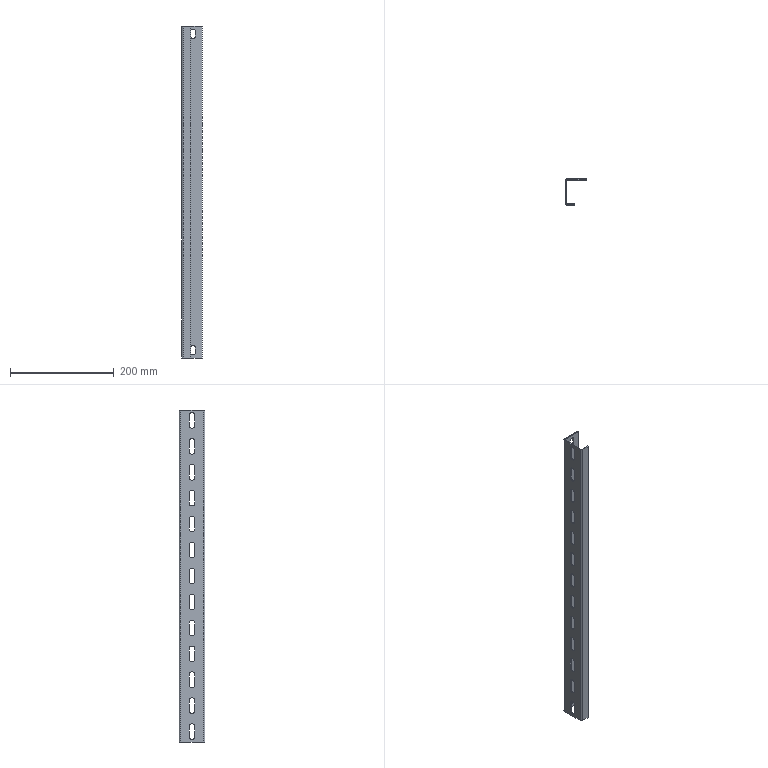Part | STEP file | 1 solid | 82 faces | box 40 x 50 x 640 mm | volume 121890 mm3 | plane 48 | cylinder 34 | commonest cylinder face diameters 11 x26 9 x4 3 x2 7 x2